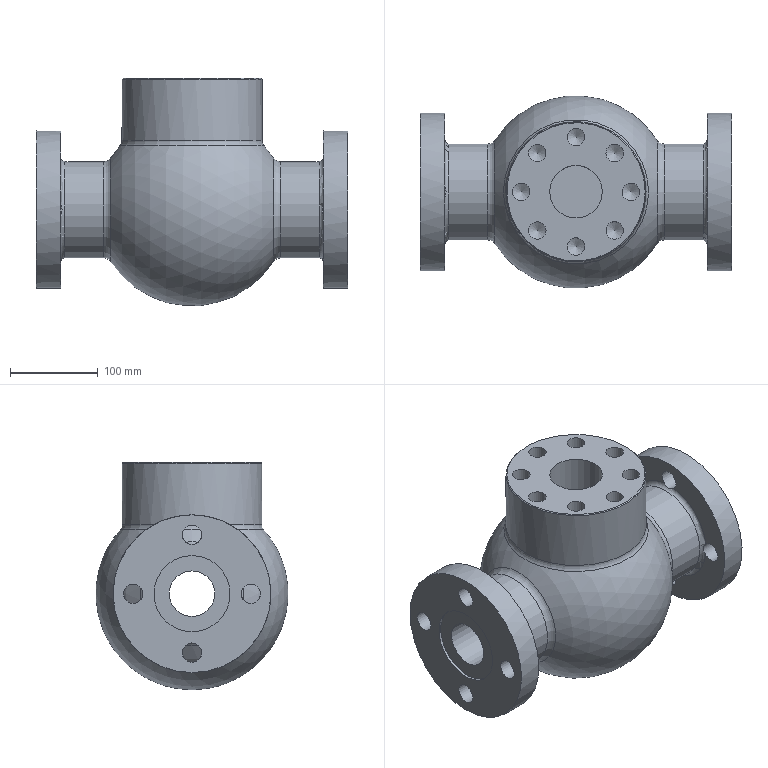Part | NX | features SIMPLE HOLE 11, SKETCH 9, DATUM_CSYS 8, EXTRACT_DATUM_AXIS 8, EXTRACT_FACE 8, HOLE PACKAGE 8, INSTANCE 8, ABSOLUTE_DATUM_AXIS 5, ABSOLUTE_DATUM_PLANE 5, SWP104 5, CHAMFER 3, Instance Feature 3, Resize Face 3, BLEND 2, AXIS_ANGLE_DATUM_PLANE 1, CIRCULAR_ISET 1, META 1, MIRROR 1, MIRROR_SET 1, Pattern Feature 1, TRANSFORM_ISET 1 | 1 solid | 48 faces | box 356 x 220 x 260 mm | volume 7990244 mm3 | cylinder 25 | cone 9 | plane 8 | torus 5 | sphere 1 | commonest cylinder face diameters 20 x8 22 x8 87 x2 110 x2 180 x2 52 x1
STEP:
#1=CARTESIAN_POINT('',(150.,0.,90.));
#2=VERTEX_POINT('',#1);
#3=CARTESIAN_POINT('',(150.,0.,0.));
#4=DIRECTION('',(-1.,0.,0.));
#5=DIRECTION('',(0.,0.,1.));
#6=AXIS2_PLACEMENT_3D('',#3,#4,#5);
#7=CIRCLE('',#6,90.);
#8=EDGE_CURVE('',#2,#2,#7,.T.);
#9=ORIENTED_EDGE('',*,*,#8,.F.);
#10=EDGE_LOOP('',(#9));
#11=FACE_BOUND('',#10,.T.);
#12=CARTESIAN_POINT('',(178.,0.,-90.));
#13=VERTEX_POINT('',#12);
#14=CARTESIAN_POINT('',(178.,0.,0.));
#15=DIRECTION('',(1.,0.,0.));
#16=DIRECTION('',(0.,0.,-1.));
#17=AXIS2_PLACEMENT_3D('',#14,#15,#16);
#18=CIRCLE('',#17,90.);
#19=EDGE_CURVE('',#13,#13,#18,.F.);
#20=ORIENTED_EDGE('',*,*,#19,.T.);
#21=EDGE_LOOP('',(#20));
#22=FACE_BOUND('',#21,.T.);
#23=CARTESIAN_POINT('',(0.,0.,0.));
#24=DIRECTION('',(1.,0.,0.));
#25=DIRECTION('',(0.,0.,-1.));
#26=AXIS2_PLACEMENT_3D('',#23,#24,#25);
#27=CYLINDRICAL_SURFACE('',#26,90.);
#28=ADVANCED_FACE('',(#11,#22),#27,.T.);
#29=CARTESIAN_POINT('',(150.,59.52,7.571));
#30=VERTEX_POINT('',#29);
#31=CARTESIAN_POINT('',(150.,59.52,-7.571));
#32=VERTEX_POINT('',#31);
#33=CARTESIAN_POINT('',(150.,67.5,0.));
#34=DIRECTION('',(-1.,0.,0.));
#35=DIRECTION('',(0.,0.,1.));
#36=AXIS2_PLACEMENT_3D('',#33,#34,#35);
#37=CIRCLE('',#36,11.);
#38=EDGE_CURVE('',#30,#32,#37,.T.);
#39=ORIENTED_EDGE('',*,*,#38,.F.);
#40=CARTESIAN_POINT('',(150.,7.571,59.52));
#41=VERTEX_POINT('',#40);
#42=CARTESIAN_POINT('',(150.,0.,0.));
#43=DIRECTION('',(-1.,0.,0.));
#44=DIRECTION('',(0.,0.,1.));
#45=AXIS2_PLACEMENT_3D('',#42,#43,#44);
#46=CIRCLE('',#45,60.);
#47=EDGE_CURVE('',#30,#41,#46,.F.);
#48=ORIENTED_EDGE('',*,*,#47,.T.);
#49=CARTESIAN_POINT('',(150.,-7.571,59.52));
#50=VERTEX_POINT('',#49);
#51=CARTESIAN_POINT('',(150.,0.,67.5));
#52=DIRECTION('',(-1.,0.,0.));
#53=DIRECTION('',(0.,0.,1.));
#54=AXIS2_PLACEMENT_3D('',#51,#52,#53);
#55=CIRCLE('',#54,11.);
#56=EDGE_CURVE('',#50,#41,#55,.T.);
#57=ORIENTED_EDGE('',*,*,#56,.F.);
#58=CARTESIAN_POINT('',(150.,-59.52,7.571));
#59=VERTEX_POINT('',#58);
#60=CARTESIAN_POINT('',(150.,0.,0.));
#61=DIRECTION('',(-1.,0.,0.));
#62=DIRECTION('',(0.,0.,1.));
#63=AXIS2_PLACEMENT_3D('',#60,#61,#62);
#64=CIRCLE('',#63,60.);
#65=EDGE_CURVE('',#50,#59,#64,.F.);
#66=ORIENTED_EDGE('',*,*,#65,.T.);
#67=CARTESIAN_POINT('',(150.,-59.52,-7.571));
#68=VERTEX_POINT('',#67);
#69=CARTESIAN_POINT('',(150.,-67.5,0.));
#70=DIRECTION('',(-1.,0.,0.));
#71=DIRECTION('',(0.,0.,1.));
#72=AXIS2_PLACEMENT_3D('',#69,#70,#71);
#73=CIRCLE('',#72,11.);
#74=EDGE_CURVE('',#68,#59,#73,.T.);
#75=ORIENTED_EDGE('',*,*,#74,.F.);
#76=CARTESIAN_POINT('',(150.,-7.571,-59.52));
#77=VERTEX_POINT('',#76);
#78=CARTESIAN_POINT('',(150.,0.,0.));
#79=DIRECTION('',(-1.,0.,0.));
#80=DIRECTION('',(0.,0.,1.));
#81=AXIS2_PLACEMENT_3D('',#78,#79,#80);
#82=CIRCLE('',#81,60.);
#83=EDGE_CURVE('',#68,#77,#82,.F.);
#84=ORIENTED_EDGE('',*,*,#83,.T.);
#85=CARTESIAN_POINT('',(150.,7.571,-59.52));
#86=VERTEX_POINT('',#85);
#87=CARTESIAN_POINT('',(150.,0.,-67.5));
#88=DIRECTION('',(-1.,0.,0.));
#89=DIRECTION('',(0.,0.,1.));
#90=AXIS2_PLACEMENT_3D('',#87,#88,#89);
#91=CIRCLE('',#90,11.);
#92=EDGE_CURVE('',#86,#77,#91,.T.);
#93=ORIENTED_EDGE('',*,*,#92,.F.);
#94=CARTESIAN_POINT('',(150.,0.,0.));
#95=DIRECTION('',(-1.,0.,0.));
#96=DIRECTION('',(0.,0.,1.));
#97=AXIS2_PLACEMENT_3D('',#94,#95,#96);
#98=CIRCLE('',#97,60.);
#99=EDGE_CURVE('',#86,#32,#98,.F.);
#100=ORIENTED_EDGE('',*,*,#99,.T.);
#101=EDGE_LOOP('',(#39,#48,#57,#66,#75,#84,#93,#100));
#102=FACE_BOUND('',#101,.T.);
#103=ORIENTED_EDGE('',*,*,#8,.T.);
#104=EDGE_LOOP('',(#103));
#105=FACE_BOUND('',#104,.T.);
#106=CARTESIAN_POINT('',(150.,0.,107.5));
#107=DIRECTION('',(-1.,0.,0.));
#108=DIRECTION('',(0.,0.,1.));
#109=AXIS2_PLACEMENT_3D('',#106,#107,#108);
#110=PLANE('',#109);
#111=ADVANCED_FACE('',(#102,#105),#110,.T.);
#112=CARTESIAN_POINT('',(-178.,0.,90.));
#113=VERTEX_POINT('',#112);
#114=CARTESIAN_POINT('',(-178.,0.,0.));
#115=DIRECTION('',(-1.,0.,0.));
#116=DIRECTION('',(0.,0.,1.));
#117=AXIS2_PLACEMENT_3D('',#114,#115,#116);
#118=CIRCLE('',#117,90.);
#119=EDGE_CURVE('',#113,#113,#118,.T.);
#120=ORIENTED_EDGE('',*,*,#119,.F.);
#121=EDGE_LOOP('',(#120));
#122=FACE_BOUND('',#121,.T.);
#123=CARTESIAN_POINT('',(-150.,0.,-90.));
#124=VERTEX_POINT('',#123);
#125=CARTESIAN_POINT('',(-150.,0.,0.));
#126=DIRECTION('',(1.,0.,0.));
#127=DIRECTION('',(0.,0.,-1.));
#128=AXIS2_PLACEMENT_3D('',#125,#126,#127);
#129=CIRCLE('',#128,90.);
#130=EDGE_CURVE('',#124,#124,#129,.F.);
#131=ORIENTED_EDGE('',*,*,#130,.T.);
#132=EDGE_LOOP('',(#131));
#133=FACE_BOUND('',#132,.T.);
#134=CARTESIAN_POINT('',(0.,0.,0.));
#135=DIRECTION('',(-1.,0.,0.));
#136=DIRECTION('',(0.,0.,-1.));
#137=AXIS2_PLACEMENT_3D('',#134,#135,#136);
#138=CYLINDRICAL_SURFACE('',#137,90.);
#139=ADVANCED_FACE('',(#122,#133),#138,.T.);
#140=CARTESIAN_POINT('',(-178.,67.2,-11.));
#141=VERTEX_POINT('',#140);
#142=CARTESIAN_POINT('',(-178.,67.2,0.));
#143=DIRECTION('',(1.,0.,0.));
#144=DIRECTION('',(0.,0.,-1.));
#145=AXIS2_PLACEMENT_3D('',#142,#143,#144);
#146=CIRCLE('',#145,11.);
#147=EDGE_CURVE('',#141,#141,#146,.T.);
#148=ORIENTED_EDGE('',*,*,#147,.T.);
#149=EDGE_LOOP('',(#148));
#150=FACE_BOUND('',#149,.T.);
#151=CARTESIAN_POINT('',(-178.,0.,-78.2));
#152=VERTEX_POINT('',#151);
#153=CARTESIAN_POINT('',(-178.,0.,-67.2));
#154=DIRECTION('',(1.,0.,0.));
#155=DIRECTION('',(0.,0.,-1.));
#156=AXIS2_PLACEMENT_3D('',#153,#154,#155);
#157=CIRCLE('',#156,11.);
#158=EDGE_CURVE('',#152,#152,#157,.T.);
#159=ORIENTED_EDGE('',*,*,#158,.T.);
#160=EDGE_LOOP('',(#159));
#161=FACE_BOUND('',#160,.T.);
#162=CARTESIAN_POINT('',(-178.,-67.2,-11.));
#163=VERTEX_POINT('',#162);
#164=CARTESIAN_POINT('',(-178.,-67.2,0.));
#165=DIRECTION('',(1.,0.,0.));
#166=DIRECTION('',(0.,0.,-1.));
#167=AXIS2_PLACEMENT_3D('',#164,#165,#166);
#168=CIRCLE('',#167,11.);
#169=EDGE_CURVE('',#163,#163,#168,.T.);
#170=ORIENTED_EDGE('',*,*,#169,.T.);
#171=EDGE_LOOP('',(#170));
#172=FACE_BOUND('',#171,.T.);
#173=CARTESIAN_POINT('',(-178.,0.,56.2));
#174=VERTEX_POINT('',#173);
#175=CARTESIAN_POINT('',(-178.,0.,67.2));
#176=DIRECTION('',(1.,0.,0.));
#177=DIRECTION('',(0.,0.,-1.));
#178=AXIS2_PLACEMENT_3D('',#175,#176,#177);
#179=CIRCLE('',#178,11.);
#180=EDGE_CURVE('',#174,#174,#179,.T.);
#181=ORIENTED_EDGE('',*,*,#180,.T.);
#182=EDGE_LOOP('',(#181));
#183=FACE_BOUND('',#182,.T.);
#184=CARTESIAN_POINT('',(-178.,0.,43.5));
#185=VERTEX_POINT('',#184);
#186=CARTESIAN_POINT('',(-178.,0.,0.));
#187=DIRECTION('',(-1.,0.,0.));
#188=DIRECTION('',(0.,0.,1.));
#189=AXIS2_PLACEMENT_3D('',#186,#187,#188);
#190=CIRCLE('',#189,43.5);
#191=EDGE_CURVE('',#185,#185,#190,.F.);
#192=ORIENTED_EDGE('',*,*,#191,.T.);
#193=EDGE_LOOP('',(#192));
#194=FACE_BOUND('',#193,.T.);
#195=ORIENTED_EDGE('',*,*,#119,.T.);
#196=EDGE_LOOP('',(#195));
#197=FACE_BOUND('',#196,.T.);
#198=CARTESIAN_POINT('',(-178.,0.,40.));
#199=DIRECTION('',(-1.,0.,0.));
#200=DIRECTION('',(0.,0.,-1.));
#201=AXIS2_PLACEMENT_3D('',#198,#199,#200);
#202=PLANE('',#201);
#203=ADVANCED_FACE('',(#150,#161,#172,#183,#194,#197),#202,.T.);
#204=CARTESIAN_POINT('',(79.,0.,150.));
#205=VERTEX_POINT('',#204);
#206=CARTESIAN_POINT('',(0.,0.,150.));
#207=DIRECTION('',(0.,0.,1.));
#208=DIRECTION('',(1.,0.,0.));
#209=AXIS2_PLACEMENT_3D('',#206,#207,#208);
#210=CIRCLE('',#209,79.);
#211=EDGE_CURVE('',#205,#205,#210,.T.);
#212=ORIENTED_EDGE('',*,*,#211,.T.);
#213=EDGE_LOOP('',(#212));
#214=FACE_BOUND('',#213,.T.);
#215=CARTESIAN_POINT('',(-69.571,7.071,150.));
#216=VERTEX_POINT('',#215);
#217=CARTESIAN_POINT('',(-62.5,0.,150.));
#218=DIRECTION('',(0.,0.,-1.));
#219=DIRECTION('',(-0.7071,0.7071,0.));
#220=AXIS2_PLACEMENT_3D('',#217,#218,#219);
#221=CIRCLE('',#220,10.);
#222=EDGE_CURVE('',#216,#216,#221,.T.);
#223=ORIENTED_EDGE('',*,*,#222,.T.);
#224=EDGE_LOOP('',(#223));
#225=FACE_BOUND('',#224,.T.);
#226=CARTESIAN_POINT('',(-44.194,54.194,150.));
#227=VERTEX_POINT('',#226);
#228=CARTESIAN_POINT('',(-44.194,44.194,150.));
#229=DIRECTION('',(0.,0.,-1.));
#230=DIRECTION('',(0.,1.,0.));
#231=AXIS2_PLACEMENT_3D('',#228,#229,#230);
#232=CIRCLE('',#231,10.);
#233=EDGE_CURVE('',#227,#227,#232,.T.);
#234=ORIENTED_EDGE('',*,*,#233,.T.);
#235=EDGE_LOOP('',(#234));
#236=FACE_BOUND('',#235,.T.);
#237=CARTESIAN_POINT('',(7.071,69.571,150.));
#238=VERTEX_POINT('',#237);
#239=CARTESIAN_POINT('',(0.,62.5,150.));
#240=DIRECTION('',(0.,0.,-1.));
#241=DIRECTION('',(0.7071,0.7071,0.));
#242=AXIS2_PLACEMENT_3D('',#239,#240,#241);
#243=CIRCLE('',#242,10.);
#244=EDGE_CURVE('',#238,#238,#243,.T.);
#245=ORIENTED_EDGE('',*,*,#244,.T.);
#246=EDGE_LOOP('',(#245));
#247=FACE_BOUND('',#246,.T.);
#248=CARTESIAN_POINT('',(54.194,44.194,150.));
#249=VERTEX_POINT('',#248);
#250=CARTESIAN_POINT('',(44.194,44.194,150.));
#251=DIRECTION('',(0.,0.,-1.));
#252=DIRECTION('',(1.,0.,0.));
#253=AXIS2_PLACEMENT_3D('',#250,#251,#252);
#254=CIRCLE('',#253,10.);
#255=EDGE_CURVE('',#249,#249,#254,.T.);
#256=ORIENTED_EDGE('',*,*,#255,.T.);
#257=EDGE_LOOP('',(#256));
#258=FACE_BOUND('',#257,.T.);
#259=CARTESIAN_POINT('',(69.571,-7.071,150.));
#260=VERTEX_POINT('',#259);
#261=CARTESIAN_POINT('',(62.5,0.,150.));
#262=DIRECTION('',(0.,0.,-1.));
#263=DIRECTION('',(0.7071,-0.7071,0.));
#264=AXIS2_PLACEMENT_3D('',#261,#262,#263);
#265=CIRCLE('',#264,10.);
#266=EDGE_CURVE('',#260,#260,#265,.T.);
#267=ORIENTED_EDGE('',*,*,#266,.T.);
#268=EDGE_LOOP('',(#267));
#269=FACE_BOUND('',#268,.T.);
#270=CARTESIAN_POINT('',(44.194,-54.194,150.));
#271=VERTEX_POINT('',#270);
#272=CARTESIAN_POINT('',(44.194,-44.194,150.));
#273=DIRECTION('',(0.,0.,-1.));
#274=DIRECTION('',(0.,-1.,0.));
#275=AXIS2_PLACEMENT_3D('',#272,#273,#274);
#276=CIRCLE('',#275,10.);
#277=EDGE_CURVE('',#271,#271,#276,.T.);
#278=ORIENTED_EDGE('',*,*,#277,.T.);
#279=EDGE_LOOP('',(#278));
#280=FACE_BOUND('',#279,.T.);
#281=CARTESIAN_POINT('',(-7.071,-69.571,150.));
#282=VERTEX_POINT('',#281);
#283=CARTESIAN_POINT('',(0.,-62.5,150.));
#284=DIRECTION('',(0.,0.,-1.));
#285=DIRECTION('',(-0.7071,-0.7071,0.));
#286=AXIS2_PLACEMENT_3D('',#283,#284,#285);
#287=CIRCLE('',#286,10.);
#288=EDGE_CURVE('',#282,#282,#287,.T.);
#289=ORIENTED_EDGE('',*,*,#288,.T.);
#290=EDGE_LOOP('',(#289));
#291=FACE_BOUND('',#290,.T.);
#292=CARTESIAN_POINT('',(-54.194,-44.194,150.));
#293=VERTEX_POINT('',#292);
#294=CARTESIAN_POINT('',(-44.194,-44.194,150.));
#295=DIRECTION('',(0.,0.,-1.));
#296=DIRECTION('',(-1.,0.,0.));
#297=AXIS2_PLACEMENT_3D('',#294,#295,#296);
#298=CIRCLE('',#297,10.);
#299=EDGE_CURVE('',#293,#293,#298,.T.);
#300=ORIENTED_EDGE('',*,*,#299,.T.);
#301=EDGE_LOOP('',(#300));
#302=FACE_BOUND('',#301,.T.);
#303=CARTESIAN_POINT('',(30.,0.,150.));
#304=VERTEX_POINT('',#303);
#305=CARTESIAN_POINT('',(0.,0.,150.));
#306=DIRECTION('',(0.,0.,1.));
#307=DIRECTION('',(1.,0.,0.));
#308=AXIS2_PLACEMENT_3D('',#305,#306,#307);
#309=CIRCLE('',#308,30.);
#310=EDGE_CURVE('',#304,#304,#309,.T.);
#311=ORIENTED_EDGE('',*,*,#310,.F.);
#312=EDGE_LOOP('',(#311));
#313=FACE_BOUND('',#312,.T.);
#314=CARTESIAN_POINT('',(0.,0.,150.));
#315=DIRECTION('',(0.,0.,1.));
#316=DIRECTION('',(1.,0.,0.));
#317=AXIS2_PLACEMENT_3D('',#314,#315,#316);
#318=PLANE('',#317);
#319=ADVANCED_FACE('',(#214,#225,#236,#247,#258,#269,#280,#291,#302,#313),#318,.T.);
#320=CARTESIAN_POINT('',(178.,67.5,11.));
#321=VERTEX_POINT('',#320);
#322=CARTESIAN_POINT('',(178.,67.5,0.));
#323=DIRECTION('',(-1.,0.,0.));
#324=DIRECTION('',(0.,0.,1.));
#325=AXIS2_PLACEMENT_3D('',#322,#323,#324);
#326=CIRCLE('',#325,11.);
#327=EDGE_CURVE('',#321,#321,#326,.T.);
#328=ORIENTED_EDGE('',*,*,#327,.T.);
#329=EDGE_LOOP('',(#328));
#330=FACE_BOUND('',#329,.T.);
#331=CARTESIAN_POINT('',(178.,0.,-56.5));
#332=VERTEX_POINT('',#331);
#333=CARTESIAN_POINT('',(178.,0.,-67.5));
#334=DIRECTION('',(-1.,0.,0.));
#335=DIRECTION('',(0.,0.,1.));
#336=AXIS2_PLACEMENT_3D('',#333,#334,#335);
#337=CIRCLE('',#336,11.);
#338=EDGE_CURVE('',#332,#332,#337,.T.);
#339=ORIENTED_EDGE('',*,*,#338,.T.);
#340=EDGE_LOOP('',(#339));
#341=FACE_BOUND('',#340,.T.);
#342=CARTESIAN_POINT('',(178.,-67.5,11.));
#343=VERTEX_POINT('',#342);
#344=CARTESIAN_POINT('',(178.,-67.5,0.));
#345=DIRECTION('',(-1.,0.,0.));
#346=DIRECTION('',(0.,0.,1.));
#347=AXIS2_PLACEMENT_3D('',#344,#345,#346);
#348=CIRCLE('',#347,11.);
#349=EDGE_CURVE('',#343,#343,#348,.T.);
#350=ORIENTED_EDGE('',*,*,#349,.T.);
#351=EDGE_LOOP('',(#350));
#352=FACE_BOUND('',#351,.T.);
#353=CARTESIAN_POINT('',(178.,0.,78.5));
#354=VERTEX_POINT('',#353);
#355=CARTESIAN_POINT('',(178.,0.,67.5));
#356=DIRECTION('',(-1.,0.,0.));
#357=DIRECTION('',(0.,0.,1.));
#358=AXIS2_PLACEMENT_3D('',#355,#356,#357);
#359=CIRCLE('',#358,11.);
#360=EDGE_CURVE('',#354,#354,#359,.T.);
#361=ORIENTED_EDGE('',*,*,#360,.T.);
#362=EDGE_LOOP('',(#361));
#363=FACE_BOUND('',#362,.T.);
#364=ORIENTED_EDGE('',*,*,#19,.F.);
#365=EDGE_LOOP('',(#364));
#366=FACE_BOUND('',#365,.T.);
#367=CARTESIAN_POINT('',(178.,0.,-43.5));
#368=VERTEX_POINT('',#367);
#369=CARTESIAN_POINT('',(178.,0.,0.));
#370=DIRECTION('',(1.,0.,0.));
#371=DIRECTION('',(0.,0.,-1.));
#372=AXIS2_PLACEMENT_3D('',#369,#370,#371);
#373=CIRCLE('',#372,43.5);
#374=EDGE_CURVE('',#368,#368,#373,.F.);
#375=ORIENTED_EDGE('',*,*,#374,.T.);
#376=EDGE_LOOP('',(#375));
#377=FACE_BOUND('',#376,.T.);
#378=CARTESIAN_POINT('',(178.,0.,40.));
#379=DIRECTION('',(1.,0.,0.));
#380=DIRECTION('',(0.,0.,-1.));
#381=AXIS2_PLACEMENT_3D('',#378,#379,#380);
#382=PLANE('',#381);
#383=ADVANCED_FACE('',(#330,#341,#352,#363,#366,#377),#382,.T.);
#384=CARTESIAN_POINT('',(100.871,0.,55.));
#385=VERTEX_POINT('',#384);
#386=CARTESIAN_POINT('',(100.871,0.,0.));
#387=DIRECTION('',(-1.,0.,0.));
#388=DIRECTION('',(0.,0.,1.));
#389=AXIS2_PLACEMENT_3D('',#386,#387,#388);
#390=CIRCLE('',#389,55.);
#391=EDGE_CURVE('',#385,#385,#390,.F.);
#392=ORIENTED_EDGE('',*,*,#391,.T.);
#393=EDGE_LOOP('',(#392));
#394=FACE_BOUND('',#393,.T.);
#395=CARTESIAN_POINT('',(145.,0.,55.));
#396=VERTEX_POINT('',#395);
#397=CARTESIAN_POINT('',(145.,0.,0.));
#398=DIRECTION('',(-1.,0.,0.));
#399=DIRECTION('',(0.,0.,1.));
#400=AXIS2_PLACEMENT_3D('',#397,#398,#399);
#401=CIRCLE('',#400,55.);
#402=EDGE_CURVE('',#396,#396,#401,.T.);
#403=ORIENTED_EDGE('',*,*,#402,.T.);
#404=EDGE_LOOP('',(#403));
#405=FACE_BOUND('',#404,.T.);
#406=CARTESIAN_POINT('',(0.,0.,0.));
#407=DIRECTION('',(1.,0.,0.));
#408=DIRECTION('',(0.,0.,-1.));
#409=AXIS2_PLACEMENT_3D('',#406,#407,#408);
#410=CYLINDRICAL_SURFACE('',#409,55.);
#411=ADVANCED_FACE('',(#394,#405),#410,.T.);
#412=CARTESIAN_POINT('',(-82.5,0.,72.758));
#413=VERTEX_POINT('',#412);
#414=CARTESIAN_POINT('',(0.,0.,72.758));
#415=DIRECTION('',(0.,0.,-1.));
#416=DIRECTION('',(-1.,0.,0.));
#417=AXIS2_PLACEMENT_3D('',#414,#415,#416);
#418=CIRCLE('',#417,82.5);
#419=EDGE_CURVE('',#413,#413,#418,.T.);
#420=ORIENTED_EDGE('',*,*,#419,.T.);
#421=EDGE_LOOP('',(#420));
#422=FACE_BOUND('',#421,.T.);
#423=CARTESIAN_POINT('',(92.465,0.,59.583));
#424=VERTEX_POINT('',#423);
#425=CARTESIAN_POINT('',(92.465,0.,0.));
#426=DIRECTION('',(-1.,0.,0.));
#427=DIRECTION('',(0.,0.,1.));
#428=AXIS2_PLACEMENT_3D('',#425,#426,#427);
#429=CIRCLE('',#428,59.583);
#430=EDGE_CURVE('',#424,#424,#429,.T.);
#431=ORIENTED_EDGE('',*,*,#430,.T.);
#432=EDGE_LOOP('',(#431));
#433=FACE_BOUND('',#432,.T.);
#434=CARTESIAN_POINT('',(-92.465,0.,-59.583));
#435=VERTEX_POINT('',#434);
#436=CARTESIAN_POINT('',(-92.465,0.,0.));
#437=DIRECTION('',(1.,0.,0.));
#438=DIRECTION('',(0.,0.,-1.));
#439=AXIS2_PLACEMENT_3D('',#436,#437,#438);
#440=CIRCLE('',#439,59.583);
#441=EDGE_CURVE('',#435,#435,#440,.T.);
#442=ORIENTED_EDGE('',*,*,#441,.T.);
#443=EDGE_LOOP('',(#442));
#444=FACE_BOUND('',#443,.T.);
#445=CARTESIAN_POINT('',(0.,0.,0.));
#446=DIRECTION('',(1.,0.,0.));
#447=DIRECTION('',(0.,0.,1.));
#448=AXIS2_PLACEMENT_3D('',#445,#446,#447);
#449=SPHERICAL_SURFACE('',#448,110.);
#450=ADVANCED_FACE('',(#422,#433,#444),#449,.T.);
#451=CARTESIAN_POINT('',(-80.,0.,79.373));
#452=VERTEX_POINT('',#451);
#453=CARTESIAN_POINT('',(0.,0.,79.373));
#454=DIRECTION('',(0.,0.,-1.));
#455=DIRECTION('',(-1.,0.,0.));
#456=AXIS2_PLACEMENT_3D('',#453,#454,#455);
#457=CIRCLE('',#456,80.);
#458=EDGE_CURVE('',#452,#452,#457,.F.);
#459=ORIENTED_EDGE('',*,*,#458,.T.);
#460=EDGE_LOOP('',(#459));
#461=FACE_BOUND('',#460,.T.);
#462=CARTESIAN_POINT('',(80.,0.,149.));
#463=VERTEX_POINT('',#462);
#464=CARTESIAN_POINT('',(0.,0.,149.));
#465=DIRECTION('',(0.,0.,1.));
#466=DIRECTION('',(1.,0.,0.));
#467=AXIS2_PLACEMENT_3D('',#464,#465,#466);
#468=CIRCLE('',#467,80.);
#469=EDGE_CURVE('',#463,#463,#468,.F.);
#470=ORIENTED_EDGE('',*,*,#469,.T.);
#471=EDGE_LOOP('',(#470));
#472=FACE_BOUND('',#471,.T.);
#473=CARTESIAN_POINT('',(0.,0.,0.));
#474=DIRECTION('',(0.,0.,1.));
#475=DIRECTION('',(1.,0.,0.));
#476=AXIS2_PLACEMENT_3D('',#473,#474,#475);
#477=CYLINDRICAL_SURFACE('',#476,80.);
#478=ADVANCED_FACE('',(#461,#472),#477,.T.);
#479=CARTESIAN_POINT('',(-150.,59.485,-7.841));
#480=VERTEX_POINT('',#479);
#481=CARTESIAN_POINT('',(-150.,59.485,7.841));
#482=VERTEX_POINT('',#481);
#483=CARTESIAN_POINT('',(-150.,67.2,0.));
#484=DIRECTION('',(1.,0.,0.));
#485=DIRECTION('',(0.,0.,-1.));
#486=AXIS2_PLACEMENT_3D('',#483,#484,#485);
#487=CIRCLE('',#486,11.);
#488=EDGE_CURVE('',#480,#482,#487,.T.);
#489=ORIENTED_EDGE('',*,*,#488,.F.);
#490=CARTESIAN_POINT('',(-150.,7.841,-59.485));
#491=VERTEX_POINT('',#490);
#492=CARTESIAN_POINT('',(-150.,0.,0.));
#493=DIRECTION('',(1.,0.,0.));
#494=DIRECTION('',(0.,0.,-1.));
#495=AXIS2_PLACEMENT_3D('',#492,#493,#494);
#496=CIRCLE('',#495,60.);
#497=EDGE_CURVE('',#480,#491,#496,.F.);
#498=ORIENTED_EDGE('',*,*,#497,.T.);
#499=CARTESIAN_POINT('',(-150.,-7.841,-59.485));
#500=VERTEX_POINT('',#499);
#501=CARTESIAN_POINT('',(-150.,0.,-67.2));
#502=DIRECTION('',(1.,0.,0.));
#503=DIRECTION('',(0.,0.,-1.));
#504=AXIS2_PLACEMENT_3D('',#501,#502,#503);
#505=CIRCLE('',#504,11.);
#506=EDGE_CURVE('',#500,#491,#505,.T.);
#507=ORIENTED_EDGE('',*,*,#506,.F.);
#508=CARTESIAN_POINT('',(-150.,-59.485,-7.841));
#509=VERTEX_POINT('',#508);
#510=CARTESIAN_POINT('',(-150.,0.,0.));
#511=DIRECTION('',(1.,0.,0.));
#512=DIRECTION('',(0.,0.,-1.));
#513=AXIS2_PLACEMENT_3D('',#510,#511,#512);
#514=CIRCLE('',#513,60.);
#515=EDGE_CURVE('',#500,#509,#514,.F.);
#516=ORIENTED_EDGE('',*,*,#515,.T.);
#517=CARTESIAN_POINT('',(-150.,-59.485,7.841));
#518=VERTEX_POINT('',#517);
#519=CARTESIAN_POINT('',(-150.,-67.2,0.));
#520=DIRECTION('',(1.,0.,0.));
#521=DIRECTION('',(0.,0.,-1.));
#522=AXIS2_PLACEMENT_3D('',#519,#520,#521);
#523=CIRCLE('',#522,11.);
#524=EDGE_CURVE('',#518,#509,#523,.T.);
#525=ORIENTED_EDGE('',*,*,#524,.F.);
#526=CARTESIAN_POINT('',(-150.,-7.841,59.485));
#527=VERTEX_POINT('',#526);
#528=CARTESIAN_POINT('',(-150.,0.,0.));
#529=DIRECTION('',(1.,0.,0.));
#530=DIRECTION('',(0.,0.,-1.));
#531=AXIS2_PLACEMENT_3D('',#528,#529,#530);
#532=CIRCLE('',#531,60.);
#533=EDGE_CURVE('',#518,#527,#532,.F.);
#534=ORIENTED_EDGE('',*,*,#533,.T.);
#535=CARTESIAN_POINT('',(-150.,7.841,59.485));
#536=VERTEX_POINT('',#535);
#537=CARTESIAN_POINT('',(-150.,0.,67.2));
#538=DIRECTION('',(1.,0.,0.));
#539=DIRECTION('',(0.,0.,-1.));
#540=AXIS2_PLACEMENT_3D('',#537,#538,#539);
#541=CIRCLE('',#540,11.);
#542=EDGE_CURVE('',#536,#527,#541,.T.);
#543=ORIENTED_EDGE('',*,*,#542,.F.);
#544=CARTESIAN_POINT('',(-150.,0.,0.));
#545=DIRECTION('',(1.,0.,0.));
#546=DIRECTION('',(0.,0.,-1.));
#547=AXIS2_PLACEMENT_3D('',#544,#545,#546);
#548=CIRCLE('',#547,60.);
#549=EDGE_CURVE('',#536,#482,#548,.F.);
#550=ORIENTED_EDGE('',*,*,#549,.T.);
#551=EDGE_LOOP('',(#489,#498,#507,#516,#525,#534,#543,#550));
#552=FACE_BOUND('',#551,.T.);
#553=ORIENTED_EDGE('',*,*,#130,.F.);
#554=EDGE_LOOP('',(#553));
#555=FACE_BOUND('',#554,.T.);
#556=CARTESIAN_POINT('',(-150.,0.,107.5));
#557=DIRECTION('',(1.,0.,0.));
#558=DIRECTION('',(0.,0.,1.));
#559=AXIS2_PLACEMENT_3D('',#556,#557,#558);
#560=PLANE('',#559);
#561=ADVANCED_FACE('',(#552,#555),#560,.T.);
#562=CARTESIAN_POINT('',(-100.871,0.,-55.));
#563=VERTEX_POINT('',#562);
#564=CARTESIAN_POINT('',(-100.871,0.,0.));
#565=DIRECTION('',(1.,0.,0.));
#566=DIRECTION('',(0.,0.,-1.));
#567=AXIS2_PLACEMENT_3D('',#564,#565,#566);
#568=CIRCLE('',#567,55.);
#569=EDGE_CURVE('',#563,#563,#568,.F.);
#570=ORIENTED_EDGE('',*,*,#569,.T.);
#571=EDGE_LOOP('',(#570));
#572=FACE_BOUND('',#571,.T.);
#573=CARTESIAN_POINT('',(-145.,0.,-55.));
#574=VERTEX_POINT('',#573);
#575=CARTESIAN_POINT('',(-145.,0.,0.));
#576=DIRECTION('',(1.,0.,0.));
#577=DIRECTION('',(0.,0.,-1.));
#578=AXIS2_PLACEMENT_3D('',#575,#576,#577);
#579=CIRCLE('',#578,55.);
#580=EDGE_CURVE('',#574,#574,#579,.T.);
#581=ORIENTED_EDGE('',*,*,#580,.T.);
#582=EDGE_LOOP('',(#581));
#583=FACE_BOUND('',#582,.T.);
#584=CARTESIAN_POINT('',(0.,0.,0.));
#585=DIRECTION('',(-1.,0.,0.));
#586=DIRECTION('',(0.,0.,-1.));
#587=AXIS2_PLACEMENT_3D('',#584,#585,#586);
#588=CYLINDRICAL_SURFACE('',#587,55.);
#589=ADVANCED_FACE('',(#572,#583),#588,.T.);
#590=CARTESIAN_POINT('',(-175.,0.,-26.));
#591=VERTEX_POINT('',#590);
#592=CARTESIAN_POINT('',(-175.,0.,0.));
#593=DIRECTION('',(1.,0.,0.));
#594=DIRECTION('',(0.,0.,-1.));
#595=AXIS2_PLACEMENT_3D('',#592,#593,#594);
#596=CIRCLE('',#595,26.);
#597=EDGE_CURVE('',#591,#591,#596,.T.);
#598=ORIENTED_EDGE('',*,*,#597,.F.);
#599=EDGE_LOOP('',(#598));
#600=FACE_BOUND('',#599,.T.);
#601=CARTESIAN_POINT('',(175.,0.,26.));
#602=VERTEX_POINT('',#601);
#603=CARTESIAN_POINT('',(175.,0.,0.));
#604=DIRECTION('',(-1.,0.,0.));
#605=DIRECTION('',(0.,0.,1.));
#606=AXIS2_PLACEMENT_3D('',#603,#604,#605);
#607=CIRCLE('',#606,26.);
#608=EDGE_CURVE('',#602,#602,#607,.T.);
#609=ORIENTED_EDGE('',*,*,#608,.F.);
#610=EDGE_LOOP('',(#609));
#611=FACE_BOUND('',#610,.T.);
#612=CARTESIAN_POINT('',(0.,0.,0.));
#613=DIRECTION('',(1.,0.,0.));
#614=DIRECTION('',(0.,0.,-1.));
#615=AXIS2_PLACEMENT_3D('',#612,#613,#614);
#616=CYLINDRICAL_SURFACE('',#615,26.);
#617=ADVANCED_FACE('',(#600,#611),#616,.F.);
#618=CARTESIAN_POINT('',(30.,0.,105.83));
#619=VERTEX_POINT('',#618);
#620=CARTESIAN_POINT('',(0.,0.,105.83));
#621=DIRECTION('',(0.,0.,1.));
#622=DIRECTION('',(1.,0.,0.));
#623=AXIS2_PLACEMENT_3D('',#620,#621,#622);
#624=CIRCLE('',#623,30.);
#625=EDGE_CURVE('',#619,#619,#624,.T.);
#626=ORIENTED_EDGE('',*,*,#625,.T.);
#627=EDGE_LOOP('',(#626));
#628=FACE_BOUND('',#627,.T.);
#629=CARTESIAN_POINT('',(0.,0.,105.83));
#630=DIRECTION('',(0.,0.,1.));
#631=DIRECTION('',(1.,0.,0.));
#632=AXIS2_PLACEMENT_3D('',#629,#630,#631);
#633=PLANE('',#632);
#634=ADVANCED_FACE('',(#628),#633,.T.);
#635=ORIENTED_EDGE('',*,*,#310,.T.);
#636=EDGE_LOOP('',(#635));
#637=FACE_BOUND('',#636,.T.);
#638=ORIENTED_EDGE('',*,*,#625,.F.);
#639=EDGE_LOOP('',(#638));
#640=FACE_BOUND('',#639,.T.);
#641=CARTESIAN_POINT('',(0.,0.,0.));
#642=DIRECTION('',(0.,0.,1.));
#643=DIRECTION('',(1.,0.,0.));
#644=AXIS2_PLACEMENT_3D('',#641,#642,#643);
#645=CYLINDRICAL_SURFACE('',#644,30.);
#646=ADVANCED_FACE('',(#637,#640),#645,.F.);
#647=CARTESIAN_POINT('',(-54.194,-44.194,130.));
#648=VERTEX_POINT('',#647);
#649=CARTESIAN_POINT('',(-44.194,-44.194,130.));
#650=DIRECTION('',(0.,0.,-1.));
#651=DIRECTION('',(-1.,0.,0.));
#652=AXIS2_PLACEMENT_3D('',#649,#650,#651);
#653=CIRCLE('',#652,10.);
#654=EDGE_CURVE('',#648,#648,#653,.T.);
#655=ORIENTED_EDGE('',*,*,#654,.F.);
#656=EDGE_LOOP('',(#655));
#657=FACE_BOUND('',#656,.T.);
#658=CARTESIAN_POINT('',(-44.194,-44.194,123.991));
#659=VERTEX_POINT('',#658);
#660=VERTEX_LOOP('',#659);
#661=FACE_BOUND('',#660,.T.);
#662=CARTESIAN_POINT('',(-44.194,-44.194,130.));
#663=DIRECTION('',(0.,0.,1.));
#664=DIRECTION('',(1.,0.,0.));
#665=AXIS2_PLACEMENT_3D('',#662,#663,#664);
#666=CONICAL_SURFACE('',#665,10.,1.03);
#667=ADVANCED_FACE('',(#657,#661),#666,.F.);
#668=ORIENTED_EDGE('',*,*,#654,.T.);
#669=EDGE_LOOP('',(#668));
#670=FACE_BOUND('',#669,.T.);
#671=ORIENTED_EDGE('',*,*,#299,.F.);
#672=EDGE_LOOP('',(#671));
#673=FACE_BOUND('',#672,.T.);
#674=CARTESIAN_POINT('',(-44.194,-44.194,150.));
#675=DIRECTION('',(0.,0.,-1.));
#676=DIRECTION('',(-1.,0.,0.));
#677=AXIS2_PLACEMENT_3D('',#674,#675,#676);
#678=CYLINDRICAL_SURFACE('',#677,10.);
#679=ADVANCED_FACE('',(#670,#673),#678,.F.);
#680=CARTESIAN_POINT('',(-7.071,-69.571,130.));
#681=VERTEX_POINT('',#680);
#682=CARTESIAN_POINT('',(0.,-62.5,130.));
#683=DIRECTION('',(0.,0.,-1.));
#684=DIRECTION('',(-0.7071,-0.7071,0.));
#685=AXIS2_PLACEMENT_3D('',#682,#683,#684);
#686=CIRCLE('',#685,10.);
#687=EDGE_CURVE('',#681,#681,#686,.T.);
#688=ORIENTED_EDGE('',*,*,#687,.F.);
#689=EDGE_LOOP('',(#688));
#690=FACE_BOUND('',#689,.T.);
#691=CARTESIAN_POINT('',(0.,-62.5,123.991));
#692=VERTEX_POINT('',#691);
#693=VERTEX_LOOP('',#692);
#694=FACE_BOUND('',#693,.T.);
#695=CARTESIAN_POINT('',(0.,-62.5,130.));
#696=DIRECTION('',(0.,0.,1.));
#697=DIRECTION('',(0.7071,0.7071,0.));
#698=AXIS2_PLACEMENT_3D('',#695,#696,#697);
#699=CONICAL_SURFACE('',#698,10.,1.03);
#700=ADVANCED_FACE('',(#690,#694),#699,.F.);
#701=ORIENTED_EDGE('',*,*,#687,.T.);
#702=EDGE_LOOP('',(#701));
#703=FACE_BOUND('',#702,.T.);
#704=ORIENTED_EDGE('',*,*,#288,.F.);
#705=EDGE_LOOP('',(#704));
#706=FACE_BOUND('',#705,.T.);
#707=CARTESIAN_POINT('',(0.,-62.5,150.));
#708=DIRECTION('',(0.,0.,-1.));
#709=DIRECTION('',(-0.7071,-0.7071,0.));
#710=AXIS2_PLACEMENT_3D('',#707,#708,#709);
#711=CYLINDRICAL_SURFACE('',#710,10.);
#712=ADVANCED_FACE('',(#703,#706),#711,.F.);
#713=CARTESIAN_POINT('',(44.194,-54.194,130.));
#714=VERTEX_POINT('',#713);
#715=CARTESIAN_POINT('',(44.194,-44.194,130.));
#716=DIRECTION('',(0.,0.,-1.));
#717=DIRECTION('',(0.,-1.,0.));
#718=AXIS2_PLACEMENT_3D('',#715,#716,#717);
#719=CIRCLE('',#718,10.);
#720=EDGE_CURVE('',#714,#714,#719,.T.);
#721=ORIENTED_EDGE('',*,*,#720,.F.);
#722=EDGE_LOOP('',(#721));
#723=FACE_BOUND('',#722,.T.);
#724=CARTESIAN_POINT('',(44.194,-44.194,123.991));
#725=VERTEX_POINT('',#724);
#726=VERTEX_LOOP('',#725);
#727=FACE_BOUND('',#726,.T.);
#728=CARTESIAN_POINT('',(44.194,-44.194,130.));
#729=DIRECTION('',(0.,0.,1.));
#730=DIRECTION('',(0.,1.,0.));
#731=AXIS2_PLACEMENT_3D('',#728,#729,#730);
#732=CONICAL_SURFACE('',#731,10.,1.03);
#733=ADVANCED_FACE('',(#723,#727),#732,.F.);
#734=ORIENTED_EDGE('',*,*,#720,.T.);
#735=EDGE_LOOP('',(#734));
#736=FACE_BOUND('',#735,.T.);
#737=ORIENTED_EDGE('',*,*,#277,.F.);
#738=EDGE_LOOP('',(#737));
#739=FACE_BOUND('',#738,.T.);
#740=CARTESIAN_POINT('',(44.194,-44.194,150.));
#741=DIRECTION('',(0.,0.,-1.));
#742=DIRECTION('',(0.,-1.,0.));
#743=AXIS2_PLACEMENT_3D('',#740,#741,#742);
#744=CYLINDRICAL_SURFACE('',#743,10.);
#745=ADVANCED_FACE('',(#736,#739),#744,.F.);
#746=CARTESIAN_POINT('',(69.571,-7.071,130.));
#747=VERTEX_POINT('',#746);
#748=CARTESIAN_POINT('',(62.5,0.,130.));
#749=DIRECTION('',(0.,0.,-1.));
#750=DIRECTION('',(0.7071,-0.7071,0.));
#751=AXIS2_PLACEMENT_3D('',#748,#749,#750);
#752=CIRCLE('',#751,10.);
#753=EDGE_CURVE('',#747,#747,#752,.T.);
#754=ORIENTED_EDGE('',*,*,#753,.F.);
#755=EDGE_LOOP('',(#754));
#756=FACE_BOUND('',#755,.T.);
#757=CARTESIAN_POINT('',(62.5,0.,123.991));
#758=VERTEX_POINT('',#757);
#759=VERTEX_LOOP('',#758);
#760=FACE_BOUND('',#759,.T.);
#761=CARTESIAN_POINT('',(62.5,0.,130.));
#762=DIRECTION('',(0.,0.,1.));
#763=DIRECTION('',(-0.7071,0.7071,0.));
#764=AXIS2_PLACEMENT_3D('',#761,#762,#763);
#765=CONICAL_SURFACE('',#764,10.,1.03);
#766=ADVANCED_FACE('',(#756,#760),#765,.F.);
#767=ORIENTED_EDGE('',*,*,#753,.T.);
#768=EDGE_LOOP('',(#767));
#769=FACE_BOUND('',#768,.T.);
#770=ORIENTED_EDGE('',*,*,#266,.F.);
#771=EDGE_LOOP('',(#770));
#772=FACE_BOUND('',#771,.T.);
#773=CARTESIAN_POINT('',(62.5,0.,150.));
#774=DIRECTION('',(0.,0.,-1.));
#775=DIRECTION('',(0.7071,-0.7071,0.));
#776=AXIS2_PLACEMENT_3D('',#773,#774,#775);
#777=CYLINDRICAL_SURFACE('',#776,10.);
#778=ADVANCED_FACE('',(#769,#772),#777,.F.);
#779=CARTESIAN_POINT('',(54.194,44.194,130.));
#780=VERTEX_POINT('',#779);
#781=CARTESIAN_POINT('',(44.194,44.194,130.));
#782=DIRECTION('',(0.,0.,-1.));
#783=DIRECTION('',(1.,0.,0.));
#784=AXIS2_PLACEMENT_3D('',#781,#782,#783);
#785=CIRCLE('',#784,10.);
#786=EDGE_CURVE('',#780,#780,#785,.T.);
#787=ORIENTED_EDGE('',*,*,#786,.F.);
#788=EDGE_LOOP('',(#787));
#789=FACE_BOUND('',#788,.T.);
#790=CARTESIAN_POINT('',(44.194,44.194,123.991));
#791=VERTEX_POINT('',#790);
#792=VERTEX_LOOP('',#791);
#793=FACE_BOUND('',#792,.T.);
#794=CARTESIAN_POINT('',(44.194,44.194,130.));
#795=DIRECTION('',(0.,0.,1.));
#796=DIRECTION('',(-1.,0.,0.));
#797=AXIS2_PLACEMENT_3D('',#794,#795,#796);
#798=CONICAL_SURFACE('',#797,10.,1.03);
#799=ADVANCED_FACE('',(#789,#793),#798,.F.);
#800=ORIENTED_EDGE('',*,*,#786,.T.);
#801=EDGE_LOOP('',(#800));
#802=FACE_BOUND('',#801,.T.);
#803=ORIENTED_EDGE('',*,*,#255,.F.);
#804=EDGE_LOOP('',(#803));
#805=FACE_BOUND('',#804,.T.);
#806=CARTESIAN_POINT('',(44.194,44.194,150.));
#807=DIRECTION('',(0.,0.,-1.));
#808=DIRECTION('',(1.,0.,0.));
#809=AXIS2_PLACEMENT_3D('',#806,#807,#808);
#810=CYLINDRICAL_SURFACE('',#809,10.);
#811=ADVANCED_FACE('',(#802,#805),#810,.F.);
#812=CARTESIAN_POINT('',(7.071,69.571,130.));
#813=VERTEX_POINT('',#812);
#814=CARTESIAN_POINT('',(0.,62.5,130.));
#815=DIRECTION('',(0.,0.,-1.));
#816=DIRECTION('',(0.7071,0.7071,0.));
#817=AXIS2_PLACEMENT_3D('',#814,#815,#816);
#818=CIRCLE('',#817,10.);
#819=EDGE_CURVE('',#813,#813,#818,.T.);
#820=ORIENTED_EDGE('',*,*,#819,.F.);
#821=EDGE_LOOP('',(#820));
#822=FACE_BOUND('',#821,.T.);
#823=CARTESIAN_POINT('',(0.,62.5,123.991));
#824=VERTEX_POINT('',#823);
#825=VERTEX_LOOP('',#824);
#826=FACE_BOUND('',#825,.T.);
#827=CARTESIAN_POINT('',(0.,62.5,130.));
#828=DIRECTION('',(0.,0.,1.));
#829=DIRECTION('',(-0.7071,-0.7071,0.));
#830=AXIS2_PLACEMENT_3D('',#827,#828,#829);
#831=CONICAL_SURFACE('',#830,10.,1.03);
#832=ADVANCED_FACE('',(#822,#826),#831,.F.);
#833=ORIENTED_EDGE('',*,*,#819,.T.);
#834=EDGE_LOOP('',(#833));
#835=FACE_BOUND('',#834,.T.);
#836=ORIENTED_EDGE('',*,*,#244,.F.);
#837=EDGE_LOOP('',(#836));
#838=FACE_BOUND('',#837,.T.);
#839=CARTESIAN_POINT('',(0.,62.5,150.));
#840=DIRECTION('',(0.,0.,-1.));
#841=DIRECTION('',(0.7071,0.7071,0.));
#842=AXIS2_PLACEMENT_3D('',#839,#840,#841);
#843=CYLINDRICAL_SURFACE('',#842,10.);
#844=ADVANCED_FACE('',(#835,#838),#843,.F.);
#845=CARTESIAN_POINT('',(-44.194,54.194,130.));
#846=VERTEX_POINT('',#845);
#847=CARTESIAN_POINT('',(-44.194,44.194,130.));
#848=DIRECTION('',(0.,0.,-1.));
#849=DIRECTION('',(0.,1.,0.));
#850=AXIS2_PLACEMENT_3D('',#847,#848,#849);
#851=CIRCLE('',#850,10.);
#852=EDGE_CURVE('',#846,#846,#851,.T.);
#853=ORIENTED_EDGE('',*,*,#852,.F.);
#854=EDGE_LOOP('',(#853));
#855=FACE_BOUND('',#854,.T.);
#856=CARTESIAN_POINT('',(-44.194,44.194,123.991));
#857=VERTEX_POINT('',#856);
#858=VERTEX_LOOP('',#857);
#859=FACE_BOUND('',#858,.T.);
#860=CARTESIAN_POINT('',(-44.194,44.194,130.));
#861=DIRECTION('',(0.,0.,1.));
#862=DIRECTION('',(0.,-1.,0.));
#863=AXIS2_PLACEMENT_3D('',#860,#861,#862);
#864=CONICAL_SURFACE('',#863,10.,1.03);
#865=ADVANCED_FACE('',(#855,#859),#864,.F.);
#866=ORIENTED_EDGE('',*,*,#852,.T.);
#867=EDGE_LOOP('',(#866));
#868=FACE_BOUND('',#867,.T.);
#869=ORIENTED_EDGE('',*,*,#233,.F.);
#870=EDGE_LOOP('',(#869));
#871=FACE_BOUND('',#870,.T.);
#872=CARTESIAN_POINT('',(-44.194,44.194,150.));
#873=DIRECTION('',(0.,0.,-1.));
#874=DIRECTION('',(0.,1.,0.));
#875=AXIS2_PLACEMENT_3D('',#872,#873,#874);
#876=CYLINDRICAL_SURFACE('',#875,10.);
#877=ADVANCED_FACE('',(#868,#871),#876,.F.);
#878=CARTESIAN_POINT('',(-69.571,7.071,130.));
#879=VERTEX_POINT('',#878);
#880=CARTESIAN_POINT('',(-62.5,0.,130.));
#881=DIRECTION('',(0.,0.,-1.));
#882=DIRECTION('',(-0.7071,0.7071,0.));
#883=AXIS2_PLACEMENT_3D('',#880,#881,#882);
#884=CIRCLE('',#883,10.);
#885=EDGE_CURVE('',#879,#879,#884,.T.);
#886=ORIENTED_EDGE('',*,*,#885,.F.);
#887=EDGE_LOOP('',(#886));
#888=FACE_BOUND('',#887,.T.);
#889=CARTESIAN_POINT('',(-62.5,0.,123.991));
#890=VERTEX_POINT('',#889);
#891=VERTEX_LOOP('',#890);
#892=FACE_BOUND('',#891,.T.);
#893=CARTESIAN_POINT('',(-62.5,0.,130.));
#894=DIRECTION('',(0.,0.,1.));
#895=DIRECTION('',(0.7071,-0.7071,0.));
#896=AXIS2_PLACEMENT_3D('',#893,#894,#895);
#897=CONICAL_SURFACE('',#896,10.,1.03);
#898=ADVANCED_FACE('',(#888,#892),#897,.F.);
#899=ORIENTED_EDGE('',*,*,#885,.T.);
#900=EDGE_LOOP('',(#899));
#901=FACE_BOUND('',#900,.T.);
#902=ORIENTED_EDGE('',*,*,#222,.F.);
#903=EDGE_LOOP('',(#902));
#904=FACE_BOUND('',#903,.T.);
#905=CARTESIAN_POINT('',(-62.5,0.,150.));
#906=DIRECTION('',(0.,0.,-1.));
#907=DIRECTION('',(-0.7071,0.7071,0.));
#908=AXIS2_PLACEMENT_3D('',#905,#906,#907);
#909=CYLINDRICAL_SURFACE('',#908,10.);
#910=ADVANCED_FACE('',(#901,#904),#909,.F.);
#911=ORIENTED_EDGE('',*,*,#608,.T.);
#912=EDGE_LOOP('',(#911));
#913=FACE_BOUND('',#912,.T.);
#914=CARTESIAN_POINT('',(175.,0.,43.5));
#915=VERTEX_POINT('',#914);
#916=CARTESIAN_POINT('',(175.,0.,0.));
#917=DIRECTION('',(-1.,0.,0.));
#918=DIRECTION('',(0.,0.,1.));
#919=AXIS2_PLACEMENT_3D('',#916,#917,#918);
#920=CIRCLE('',#919,43.5);
#921=EDGE_CURVE('',#915,#915,#920,.T.);
#922=ORIENTED_EDGE('',*,*,#921,.F.);
#923=EDGE_LOOP('',(#922));
#924=FACE_BOUND('',#923,.T.);
#925=CARTESIAN_POINT('',(175.,0.,0.));
#926=DIRECTION('',(-1.,0.,0.));
#927=DIRECTION('',(0.,0.,1.));
#928=AXIS2_PLACEMENT_3D('',#925,#926,#927);
#929=PLANE('',#928);
#930=ADVANCED_FACE('',(#913,#924),#929,.F.);
#931=ORIENTED_EDGE('',*,*,#921,.T.);
#932=EDGE_LOOP('',(#931));
#933=FACE_BOUND('',#932,.T.);
#934=ORIENTED_EDGE('',*,*,#374,.F.);
#935=EDGE_LOOP('',(#934));
#936=FACE_BOUND('',#935,.T.);
#937=CARTESIAN_POINT('',(178.,0.,0.));
#938=DIRECTION('',(-1.,0.,0.));
#939=DIRECTION('',(0.,0.,1.));
#940=AXIS2_PLACEMENT_3D('',#937,#938,#939);
#941=CYLINDRICAL_SURFACE('',#940,43.5);
#942=ADVANCED_FACE('',(#933,#936),#941,.F.);
#943=ORIENTED_EDGE('',*,*,#597,.T.);
#944=EDGE_LOOP('',(#943));
#945=FACE_BOUND('',#944,.T.);
#946=CARTESIAN_POINT('',(-175.,0.,-43.5));
#947=VERTEX_POINT('',#946);
#948=CARTESIAN_POINT('',(-175.,0.,0.));
#949=DIRECTION('',(1.,0.,0.));
#950=DIRECTION('',(0.,0.,-1.));
#951=AXIS2_PLACEMENT_3D('',#948,#949,#950);
#952=CIRCLE('',#951,43.5);
#953=EDGE_CURVE('',#947,#947,#952,.T.);
#954=ORIENTED_EDGE('',*,*,#953,.F.);
#955=EDGE_LOOP('',(#954));
#956=FACE_BOUND('',#955,.T.);
#957=CARTESIAN_POINT('',(-175.,0.,0.));
#958=DIRECTION('',(1.,0.,0.));
#959=DIRECTION('',(0.,0.,-1.));
#960=AXIS2_PLACEMENT_3D('',#957,#958,#959);
#961=PLANE('',#960);
#962=ADVANCED_FACE('',(#945,#956),#961,.F.);
#963=ORIENTED_EDGE('',*,*,#953,.T.);
#964=EDGE_LOOP('',(#963));
#965=FACE_BOUND('',#964,.T.);
#966=ORIENTED_EDGE('',*,*,#191,.F.);
#967=EDGE_LOOP('',(#966));
#968=FACE_BOUND('',#967,.T.);
#969=CARTESIAN_POINT('',(-178.,0.,0.));
#970=DIRECTION('',(1.,0.,0.));
#971=DIRECTION('',(0.,0.,-1.));
#972=AXIS2_PLACEMENT_3D('',#969,#970,#971);
#973=CYLINDRICAL_SURFACE('',#972,43.5);
#974=ADVANCED_FACE('',(#965,#968),#973,.F.);
#975=ORIENTED_EDGE('',*,*,#497,.F.);
#976=CARTESIAN_POINT('',(-150.,59.485,-7.841));
#977=CARTESIAN_POINT('',(-150.,58.425,-6.798));
#978=CARTESIAN_POINT('',(-149.382,57.199,-4.951));
#979=CARTESIAN_POINT('',(-148.48,56.354,-2.227));
#980=CARTESIAN_POINT('',(-148.134,56.122,0.006429));
#981=CARTESIAN_POINT('',(-148.484,56.357,2.238));
#982=CARTESIAN_POINT('',(-149.381,57.201,4.95));
#983=CARTESIAN_POINT('',(-150.,58.412,6.785));
#984=CARTESIAN_POINT('',(-150.,59.485,7.841));
#985=B_SPLINE_CURVE_WITH_KNOTS('',3,(#976,#977,#978,#979,#980,#981,#982,#983,#984),.UNSPECIFIED.,.F.,.F.,(4,1,1,1,1,1,4),(0.0006948,0.005144,0.007369,0.009593,0.01182,0.01404,0.01849),.UNSPECIFIED.);
#986=EDGE_CURVE('',#480,#482,#985,.T.);
#987=ORIENTED_EDGE('',*,*,#986,.T.);
#988=ORIENTED_EDGE('',*,*,#549,.F.);
#989=CARTESIAN_POINT('',(-150.,7.841,59.485));
#990=CARTESIAN_POINT('',(-150.,6.798,58.425));
#991=CARTESIAN_POINT('',(-149.382,4.951,57.199));
#992=CARTESIAN_POINT('',(-148.48,2.227,56.354));
#993=CARTESIAN_POINT('',(-148.134,-0.006429,56.122));
#994=CARTESIAN_POINT('',(-148.484,-2.238,56.357));
#995=CARTESIAN_POINT('',(-149.381,-4.95,57.201));
#996=CARTESIAN_POINT('',(-150.,-6.785,58.412));
#997=CARTESIAN_POINT('',(-150.,-7.841,59.485));
#998=B_SPLINE_CURVE_WITH_KNOTS('',3,(#989,#990,#991,#992,#993,#994,#995,#996,#997),.UNSPECIFIED.,.F.,.F.,(4,1,1,1,1,1,4),(0.0006948,0.005144,0.007369,0.009593,0.01182,0.01404,0.01849),.UNSPECIFIED.);
#999=EDGE_CURVE('',#536,#527,#998,.T.);
#1000=ORIENTED_EDGE('',*,*,#999,.T.);
#1001=ORIENTED_EDGE('',*,*,#533,.F.);
#1002=CARTESIAN_POINT('',(-150.,-59.485,7.841));
#1003=CARTESIAN_POINT('',(-150.,-58.425,6.798));
#1004=CARTESIAN_POINT('',(-149.382,-57.199,4.951));
#1005=CARTESIAN_POINT('',(-148.48,-56.354,2.227));
#1006=CARTESIAN_POINT('',(-148.134,-56.122,-0.006429));
#1007=CARTESIAN_POINT('',(-148.484,-56.357,-2.238));
#1008=CARTESIAN_POINT('',(-149.381,-57.201,-4.95));
#1009=CARTESIAN_POINT('',(-150.,-58.412,-6.785));
#1010=CARTESIAN_POINT('',(-150.,-59.485,-7.841));
#1011=B_SPLINE_CURVE_WITH_KNOTS('',3,(#1002,#1003,#1004,#1005,#1006,#1007,#1008,#1009,#1010),.UNSPECIFIED.,.F.,.F.,(4,1,1,1,1,1,4),(0.0006948,0.005144,0.007369,0.009593,0.01182,0.01404,0.01849),.UNSPECIFIED.);
#1012=EDGE_CURVE('',#518,#509,#1011,.T.);
#1013=ORIENTED_EDGE('',*,*,#1012,.T.);
#1014=ORIENTED_EDGE('',*,*,#515,.F.);
#1015=CARTESIAN_POINT('',(-150.,-7.841,-59.485));
#1016=CARTESIAN_POINT('',(-150.,-6.798,-58.425));
#1017=CARTESIAN_POINT('',(-149.382,-4.951,-57.199));
#1018=CARTESIAN_POINT('',(-148.48,-2.227,-56.354));
#1019=CARTESIAN_POINT('',(-148.134,0.006429,-56.122));
#1020=CARTESIAN_POINT('',(-148.484,2.238,-56.357));
#1021=CARTESIAN_POINT('',(-149.381,4.95,-57.201));
#1022=CARTESIAN_POINT('',(-150.,6.785,-58.412));
#1023=CARTESIAN_POINT('',(-150.,7.841,-59.485));
#1024=B_SPLINE_CURVE_WITH_KNOTS('',3,(#1015,#1016,#1017,#1018,#1019,#1020,#1021,#1022,#1023),.UNSPECIFIED.,.F.,.F.,(4,1,1,1,1,1,4),(0.0006948,0.005144,0.007369,0.009593,0.01182,0.01404,0.01849),.UNSPECIFIED.);
#1025=EDGE_CURVE('',#500,#491,#1024,.T.);
#1026=ORIENTED_EDGE('',*,*,#1025,.T.);
#1027=EDGE_LOOP('',(#975,#987,#988,#1000,#1001,#1013,#1014,#1026));
#1028=FACE_BOUND('',#1027,.T.);
#1029=ORIENTED_EDGE('',*,*,#580,.F.);
#1030=EDGE_LOOP('',(#1029));
#1031=FACE_BOUND('',#1030,.T.);
#1032=CARTESIAN_POINT('',(-145.,0.,0.));
#1033=DIRECTION('',(1.,0.,0.));
#1034=DIRECTION('',(0.,0.,-1.));
#1035=AXIS2_PLACEMENT_3D('',#1032,#1033,#1034);
#1036=TOROIDAL_SURFACE('',#1035,60.,5.);
#1037=ADVANCED_FACE('',(#1028,#1031),#1036,.F.);
#1038=ORIENTED_EDGE('',*,*,#402,.F.);
#1039=EDGE_LOOP('',(#1038));
#1040=FACE_BOUND('',#1039,.T.);
#1041=ORIENTED_EDGE('',*,*,#47,.F.);
#1042=CARTESIAN_POINT('',(150.,59.52,7.571));
#1043=CARTESIAN_POINT('',(150.,58.545,6.544));
#1044=CARTESIAN_POINT('',(149.29,57.043,4.185));
#1045=CARTESIAN_POINT('',(148.211,56.228,-0.01226));
#1046=CARTESIAN_POINT('',(149.292,57.046,-4.186));
#1047=CARTESIAN_POINT('',(150.,58.547,-6.545));
#1048=CARTESIAN_POINT('',(150.,59.52,-7.571));
#1049=B_SPLINE_CURVE_WITH_KNOTS('',3,(#1042,#1043,#1044,#1045,#1046,#1047,#1048),.UNSPECIFIED.,.F.,.F.,(4,1,1,1,4),(0.0006703,0.004906,0.009142,0.01338,0.01761),.UNSPECIFIED.);
#1050=EDGE_CURVE('',#30,#32,#1049,.T.);
#1051=ORIENTED_EDGE('',*,*,#1050,.T.);
#1052=ORIENTED_EDGE('',*,*,#99,.F.);
#1053=CARTESIAN_POINT('',(150.,7.571,-59.52));
#1054=CARTESIAN_POINT('',(150.,6.544,-58.545));
#1055=CARTESIAN_POINT('',(149.29,4.185,-57.043));
#1056=CARTESIAN_POINT('',(148.211,-0.01226,-56.228));
#1057=CARTESIAN_POINT('',(149.292,-4.186,-57.046));
#1058=CARTESIAN_POINT('',(150.,-6.545,-58.547));
#1059=CARTESIAN_POINT('',(150.,-7.571,-59.52));
#1060=B_SPLINE_CURVE_WITH_KNOTS('',3,(#1053,#1054,#1055,#1056,#1057,#1058,#1059),.UNSPECIFIED.,.F.,.F.,(4,1,1,1,4),(0.0006703,0.004906,0.009142,0.01338,0.01761),.UNSPECIFIED.);
#1061=EDGE_CURVE('',#86,#77,#1060,.T.);
#1062=ORIENTED_EDGE('',*,*,#1061,.T.);
#1063=ORIENTED_EDGE('',*,*,#83,.F.);
#1064=CARTESIAN_POINT('',(150.,-59.52,-7.571));
#1065=CARTESIAN_POINT('',(150.,-58.545,-6.544));
#1066=CARTESIAN_POINT('',(149.29,-57.043,-4.185));
#1067=CARTESIAN_POINT('',(148.211,-56.228,0.01226));
#1068=CARTESIAN_POINT('',(149.292,-57.046,4.186));
#1069=CARTESIAN_POINT('',(150.,-58.547,6.545));
#1070=CARTESIAN_POINT('',(150.,-59.52,7.571));
#1071=B_SPLINE_CURVE_WITH_KNOTS('',3,(#1064,#1065,#1066,#1067,#1068,#1069,#1070),.UNSPECIFIED.,.F.,.F.,(4,1,1,1,4),(0.0006703,0.004906,0.009142,0.01338,0.01761),.UNSPECIFIED.);
#1072=EDGE_CURVE('',#68,#59,#1071,.T.);
#1073=ORIENTED_EDGE('',*,*,#1072,.T.);
#1074=ORIENTED_EDGE('',*,*,#65,.F.);
#1075=CARTESIAN_POINT('',(150.,-7.571,59.52));
#1076=CARTESIAN_POINT('',(150.,-6.544,58.545));
#1077=CARTESIAN_POINT('',(149.29,-4.185,57.043));
#1078=CARTESIAN_POINT('',(148.211,0.01226,56.228));
#1079=CARTESIAN_POINT('',(149.292,4.186,57.046));
#1080=CARTESIAN_POINT('',(150.,6.545,58.547));
#1081=CARTESIAN_POINT('',(150.,7.571,59.52));
#1082=B_SPLINE_CURVE_WITH_KNOTS('',3,(#1075,#1076,#1077,#1078,#1079,#1080,#1081),.UNSPECIFIED.,.F.,.F.,(4,1,1,1,4),(0.0006703,0.004906,0.009142,0.01338,0.01761),.UNSPECIFIED.);
#1083=EDGE_CURVE('',#50,#41,#1082,.T.);
#1084=ORIENTED_EDGE('',*,*,#1083,.T.);
#1085=EDGE_LOOP('',(#1041,#1051,#1052,#1062,#1063,#1073,#1074,#1084));
#1086=FACE_BOUND('',#1085,.T.);
#1087=CARTESIAN_POINT('',(145.,0.,0.));
#1088=DIRECTION('',(-1.,0.,0.));
#1089=DIRECTION('',(0.,0.,1.));
#1090=AXIS2_PLACEMENT_3D('',#1087,#1088,#1089);
#1091=TOROIDAL_SURFACE('',#1090,60.,5.);
#1092=ADVANCED_FACE('',(#1040,#1086),#1091,.F.);
#1093=ORIENTED_EDGE('',*,*,#469,.F.);
#1094=EDGE_LOOP('',(#1093));
#1095=FACE_BOUND('',#1094,.T.);
#1096=ORIENTED_EDGE('',*,*,#211,.F.);
#1097=EDGE_LOOP('',(#1096));
#1098=FACE_BOUND('',#1097,.T.);
#1099=CARTESIAN_POINT('',(0.,0.,150.));
#1100=DIRECTION('',(0.,0.,-1.));
#1101=DIRECTION('',(-1.,0.,0.));
#1102=AXIS2_PLACEMENT_3D('',#1099,#1100,#1101);
#1103=CONICAL_SURFACE('',#1102,79.,0.7854);
#1104=ADVANCED_FACE('',(#1095,#1098),#1103,.T.);
#1105=ORIENTED_EDGE('',*,*,#419,.F.);
#1106=EDGE_LOOP('',(#1105));
#1107=FACE_BOUND('',#1106,.T.);
#1108=ORIENTED_EDGE('',*,*,#458,.F.);
#1109=EDGE_LOOP('',(#1108));
#1110=FACE_BOUND('',#1109,.T.);
#1111=CARTESIAN_POINT('',(0.,0.,79.373));
#1112=DIRECTION('',(0.,0.,-1.));
#1113=DIRECTION('',(-1.,0.,0.));
#1114=AXIS2_PLACEMENT_3D('',#1111,#1112,#1113);
#1115=TOROIDAL_SURFACE('',#1114,90.,10.);
#1116=ADVANCED_FACE('',(#1107,#1110),#1115,.F.);
#1117=ORIENTED_EDGE('',*,*,#430,.F.);
#1118=EDGE_LOOP('',(#1117));
#1119=FACE_BOUND('',#1118,.T.);
#1120=ORIENTED_EDGE('',*,*,#391,.F.);
#1121=EDGE_LOOP('',(#1120));
#1122=FACE_BOUND('',#1121,.T.);
#1123=CARTESIAN_POINT('',(100.871,0.,0.));
#1124=DIRECTION('',(-1.,0.,0.));
#1125=DIRECTION('',(0.,0.,1.));
#1126=AXIS2_PLACEMENT_3D('',#1123,#1124,#1125);
#1127=TOROIDAL_SURFACE('',#1126,65.,10.);
#1128=ADVANCED_FACE('',(#1119,#1122),#1127,.F.);
#1129=ORIENTED_EDGE('',*,*,#569,.F.);
#1130=EDGE_LOOP('',(#1129));
#1131=FACE_BOUND('',#1130,.T.);
#1132=ORIENTED_EDGE('',*,*,#441,.F.);
#1133=EDGE_LOOP('',(#1132));
#1134=FACE_BOUND('',#1133,.T.);
#1135=CARTESIAN_POINT('',(-100.871,0.,0.));
#1136=DIRECTION('',(1.,0.,0.));
#1137=DIRECTION('',(0.,0.,-1.));
#1138=AXIS2_PLACEMENT_3D('',#1135,#1136,#1137);
#1139=TOROIDAL_SURFACE('',#1138,65.,10.);
#1140=ADVANCED_FACE('',(#1131,#1134),#1139,.F.);
#1141=ORIENTED_EDGE('',*,*,#56,.T.);
#1142=ORIENTED_EDGE('',*,*,#1083,.F.);
#1143=EDGE_LOOP('',(#1141,#1142));
#1144=FACE_BOUND('',#1143,.T.);
#1145=ORIENTED_EDGE('',*,*,#360,.F.);
#1146=EDGE_LOOP('',(#1145));
#1147=FACE_BOUND('',#1146,.T.);
#1148=CARTESIAN_POINT('',(178.,0.,67.5));
#1149=DIRECTION('',(-1.,0.,0.));
#1150=DIRECTION('',(0.,0.,1.));
#1151=AXIS2_PLACEMENT_3D('',#1148,#1149,#1150);
#1152=CYLINDRICAL_SURFACE('',#1151,11.);
#1153=ADVANCED_FACE('',(#1144,#1147),#1152,.F.);
#1154=ORIENTED_EDGE('',*,*,#542,.T.);
#1155=ORIENTED_EDGE('',*,*,#999,.F.);
#1156=EDGE_LOOP('',(#1154,#1155));
#1157=FACE_BOUND('',#1156,.T.);
#1158=ORIENTED_EDGE('',*,*,#180,.F.);
#1159=EDGE_LOOP('',(#1158));
#1160=FACE_BOUND('',#1159,.T.);
#1161=CARTESIAN_POINT('',(-178.,0.,67.2));
#1162=DIRECTION('',(1.,0.,0.));
#1163=DIRECTION('',(0.,0.,-1.));
#1164=AXIS2_PLACEMENT_3D('',#1161,#1162,#1163);
#1165=CYLINDRICAL_SURFACE('',#1164,11.);
#1166=ADVANCED_FACE('',(#1157,#1160),#1165,.F.);
#1167=ORIENTED_EDGE('',*,*,#74,.T.);
#1168=ORIENTED_EDGE('',*,*,#1072,.F.);
#1169=EDGE_LOOP('',(#1167,#1168));
#1170=FACE_BOUND('',#1169,.T.);
#1171=ORIENTED_EDGE('',*,*,#349,.F.);
#1172=EDGE_LOOP('',(#1171));
#1173=FACE_BOUND('',#1172,.T.);
#1174=CARTESIAN_POINT('',(178.,-67.5,0.));
#1175=DIRECTION('',(-1.,0.,0.));
#1176=DIRECTION('',(0.,0.,1.));
#1177=AXIS2_PLACEMENT_3D('',#1174,#1175,#1176);
#1178=CYLINDRICAL_SURFACE('',#1177,11.);
#1179=ADVANCED_FACE('',(#1170,#1173),#1178,.F.);
#1180=ORIENTED_EDGE('',*,*,#524,.T.);
#1181=ORIENTED_EDGE('',*,*,#1012,.F.);
#1182=EDGE_LOOP('',(#1180,#1181));
#1183=FACE_BOUND('',#1182,.T.);
#1184=ORIENTED_EDGE('',*,*,#169,.F.);
#1185=EDGE_LOOP('',(#1184));
#1186=FACE_BOUND('',#1185,.T.);
#1187=CARTESIAN_POINT('',(-178.,-67.2,0.));
#1188=DIRECTION('',(1.,0.,0.));
#1189=DIRECTION('',(0.,0.,-1.));
#1190=AXIS2_PLACEMENT_3D('',#1187,#1188,#1189);
#1191=CYLINDRICAL_SURFACE('',#1190,11.);
#1192=ADVANCED_FACE('',(#1183,#1186),#1191,.F.);
#1193=ORIENTED_EDGE('',*,*,#92,.T.);
#1194=ORIENTED_EDGE('',*,*,#1061,.F.);
#1195=EDGE_LOOP('',(#1193,#1194));
#1196=FACE_BOUND('',#1195,.T.);
#1197=ORIENTED_EDGE('',*,*,#338,.F.);
#1198=EDGE_LOOP('',(#1197));
#1199=FACE_BOUND('',#1198,.T.);
#1200=CARTESIAN_POINT('',(178.,0.,-67.5));
#1201=DIRECTION('',(-1.,0.,0.));
#1202=DIRECTION('',(0.,0.,1.));
#1203=AXIS2_PLACEMENT_3D('',#1200,#1201,#1202);
#1204=CYLINDRICAL_SURFACE('',#1203,11.);
#1205=ADVANCED_FACE('',(#1196,#1199),#1204,.F.);
#1206=ORIENTED_EDGE('',*,*,#506,.T.);
#1207=ORIENTED_EDGE('',*,*,#1025,.F.);
#1208=EDGE_LOOP('',(#1206,#1207));
#1209=FACE_BOUND('',#1208,.T.);
#1210=ORIENTED_EDGE('',*,*,#158,.F.);
#1211=EDGE_LOOP('',(#1210));
#1212=FACE_BOUND('',#1211,.T.);
#1213=CARTESIAN_POINT('',(-178.,0.,-67.2));
#1214=DIRECTION('',(1.,0.,0.));
#1215=DIRECTION('',(0.,0.,-1.));
#1216=AXIS2_PLACEMENT_3D('',#1213,#1214,#1215);
#1217=CYLINDRICAL_SURFACE('',#1216,11.);
#1218=ADVANCED_FACE('',(#1209,#1212),#1217,.F.);
#1219=ORIENTED_EDGE('',*,*,#38,.T.);
#1220=ORIENTED_EDGE('',*,*,#1050,.F.);
#1221=EDGE_LOOP('',(#1219,#1220));
#1222=FACE_BOUND('',#1221,.T.);
#1223=ORIENTED_EDGE('',*,*,#327,.F.);
#1224=EDGE_LOOP('',(#1223));
#1225=FACE_BOUND('',#1224,.T.);
#1226=CARTESIAN_POINT('',(178.,67.5,0.));
#1227=DIRECTION('',(-1.,0.,0.));
#1228=DIRECTION('',(0.,0.,1.));
#1229=AXIS2_PLACEMENT_3D('',#1226,#1227,#1228);
#1230=CYLINDRICAL_SURFACE('',#1229,11.);
#1231=ADVANCED_FACE('',(#1222,#1225),#1230,.F.);
#1232=ORIENTED_EDGE('',*,*,#488,.T.);
#1233=ORIENTED_EDGE('',*,*,#986,.F.);
#1234=EDGE_LOOP('',(#1232,#1233));
#1235=FACE_BOUND('',#1234,.T.);
#1236=ORIENTED_EDGE('',*,*,#147,.F.);
#1237=EDGE_LOOP('',(#1236));
#1238=FACE_BOUND('',#1237,.T.);
#1239=CARTESIAN_POINT('',(-178.,67.2,0.));
#1240=DIRECTION('',(1.,0.,0.));
#1241=DIRECTION('',(0.,0.,-1.));
#1242=AXIS2_PLACEMENT_3D('',#1239,#1240,#1241);
#1243=CYLINDRICAL_SURFACE('',#1242,11.);
#1244=ADVANCED_FACE('',(#1235,#1238),#1243,.F.);
#1245=CLOSED_SHELL('',(#28,#111,#139,#203,#319,#383,#411,#450,#478,#561,#589,#617,#634,#646,#667,#679,#700,#712,#733,#745,#766,#778,#799,#811,#832,#844,#865,#877,#898,#910,#930,#942,#962,#974,#1037,#1092,#1104,#1116,#1128,#1140,#1153,#1166,#1179,#1192,#1205,#1218,#1231,#1244));
#1246=MANIFOLD_SOLID_BREP('',#1245);
#1247=(LENGTH_UNIT()NAMED_UNIT(*)SI_UNIT(.MILLI.,.METRE.));
#1248=UNCERTAINTY_MEASURE_WITH_UNIT(LENGTH_MEASURE(0.0508),#1247,'','');
#1249=(NAMED_UNIT(*)PLANE_ANGLE_UNIT()SI_UNIT($,.RADIAN.));
#1250=(NAMED_UNIT(*)SI_UNIT($,.STERADIAN.)SOLID_ANGLE_UNIT());
#1251=(GEOMETRIC_REPRESENTATION_CONTEXT(3)GLOBAL_UNCERTAINTY_ASSIGNED_CONTEXT((#1248))GLOBAL_UNIT_ASSIGNED_CONTEXT((#1247,#1249,#1250))REPRESENTATION_CONTEXT('',''));
#1252=ADVANCED_BREP_SHAPE_REPRESENTATION('',(#1246),#1251);